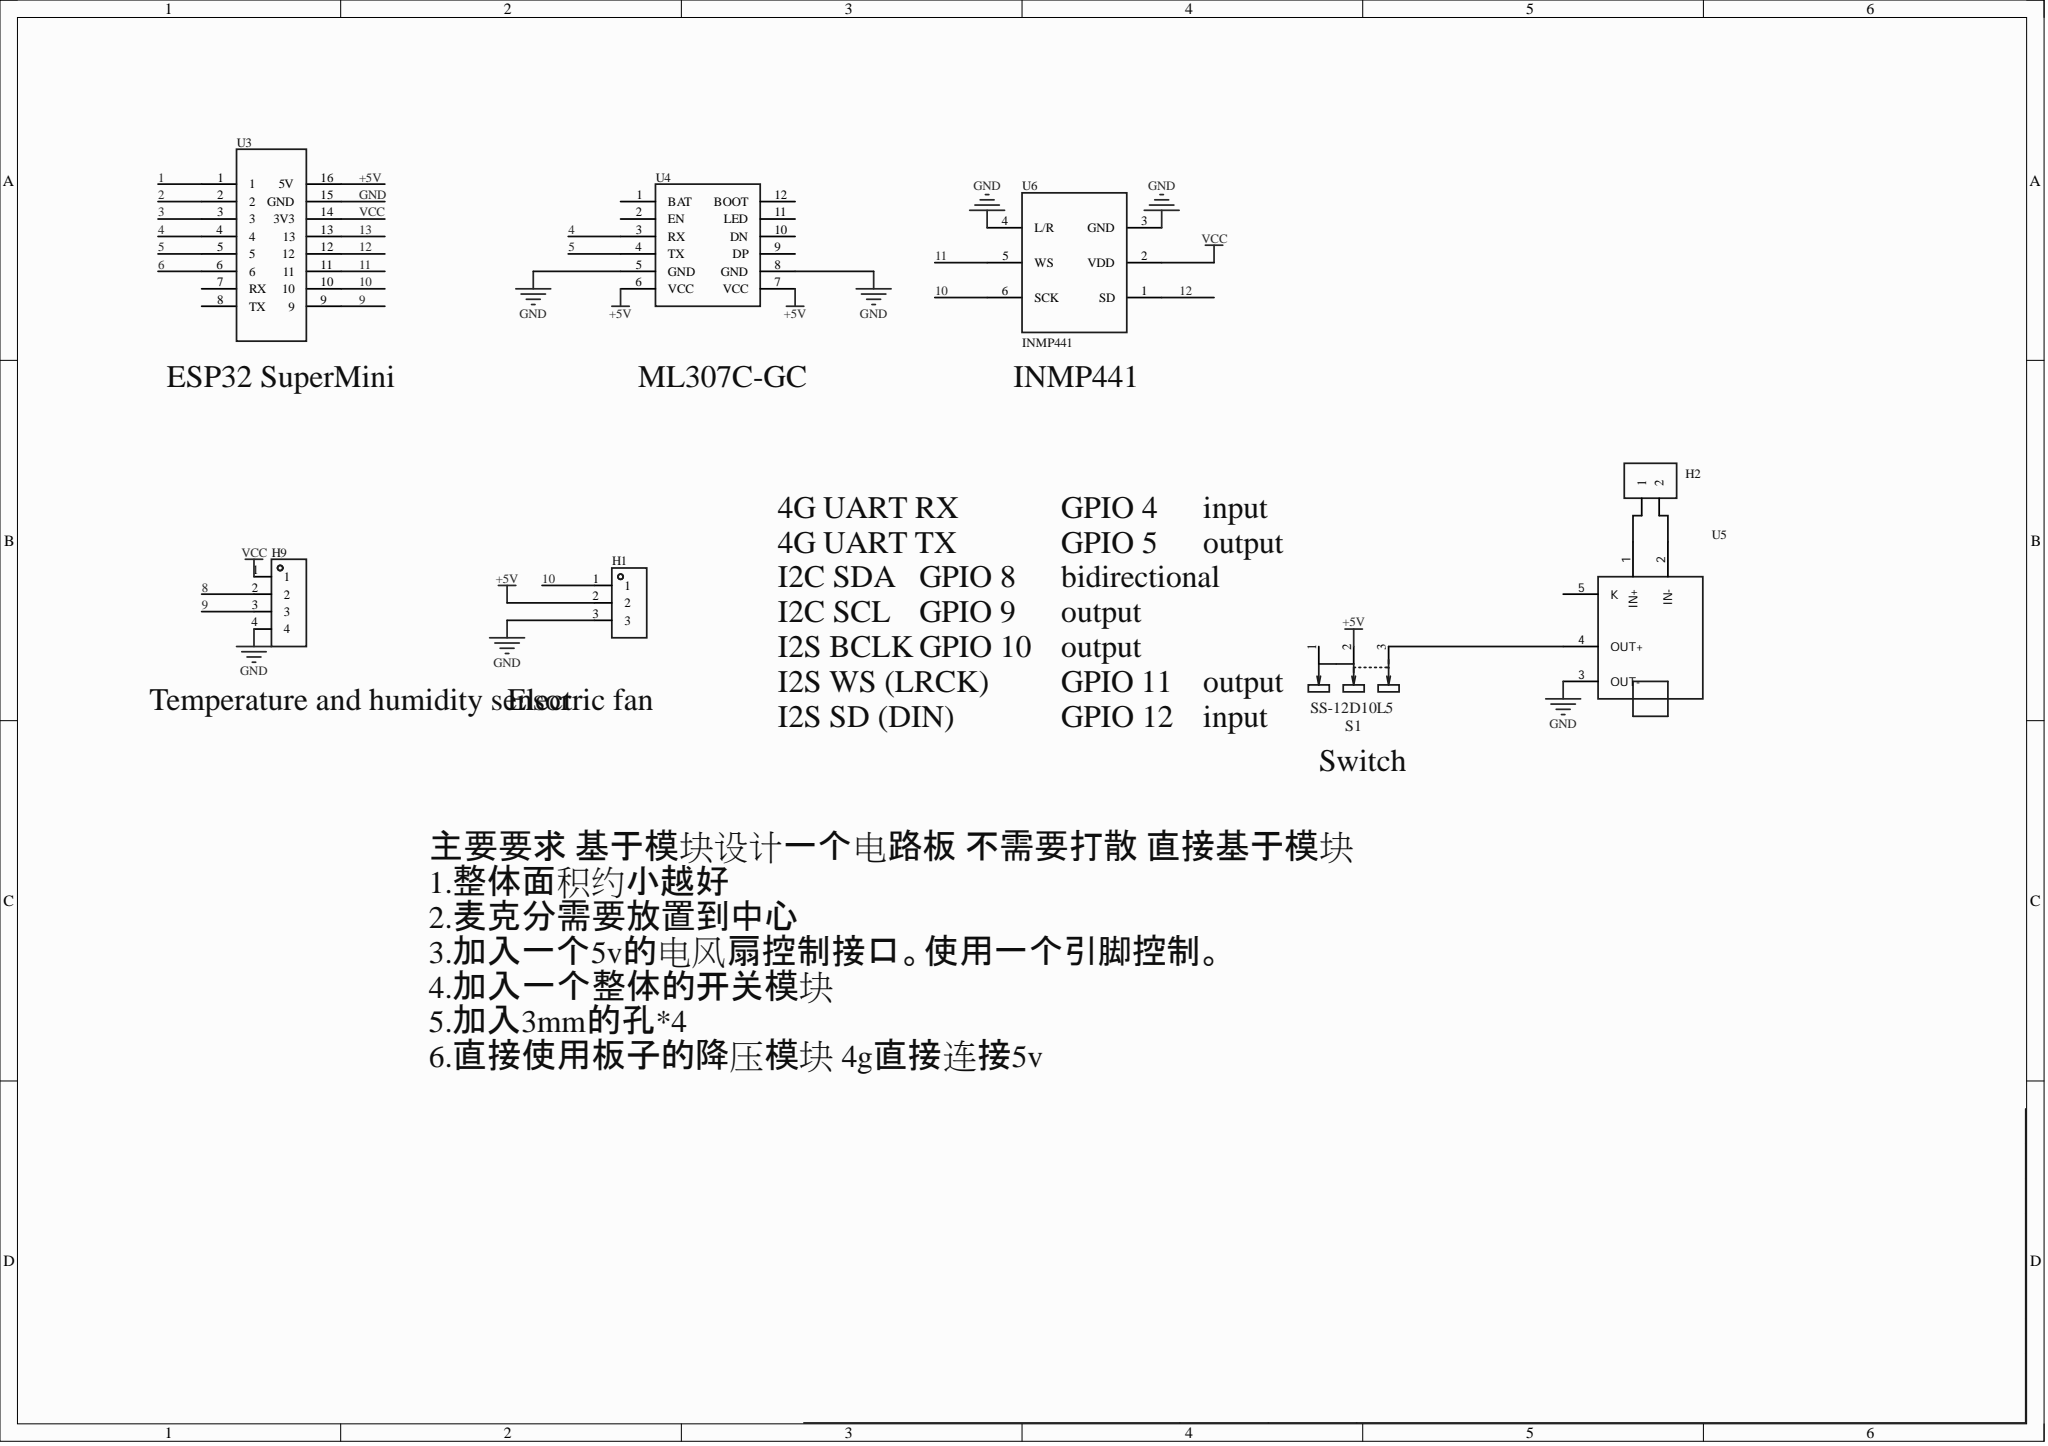Circuit board | Altium Designer | 8 parts | 12 nets
Bill of materials:
Comment,Description,Designator,Footprint,LibRef,Quantity
"","","H1","HDR-TH_3P-P2.54-V-M","HDR-M_2.54_1x3P","1"
"","","H2","HDR-TH_2P-P2.54-V-F","HDR-F_2.54_1x2P","1"
"","","H9","HDR-TH_4P-P2.54-V-F","HDR-F_2.54_1x4P","1"
"SS-12D10L5","","S1","SS-12D10L5","SS-12D10L5","1"
"","","U3","【封装Supermini】","ESP32 SuperMini","1"
"","","U4","ML307C-GC核心板","ML307C-GC核心板","1"
"","","U5","5V2A充放电一体模块","5V2A充放电一体模块","1"
"INMP441","","U6","INMP441","INMP441","1"
Netlist (Protel format):
[
H1
HDR-TH_3P-P2.54-V-M




]
[
H2
HDR-TH_2P-P2.54-V-F




]
[
H9
HDR-TH_4P-P2.54-V-F




]
[
S1
SS-12D10L5
SS-12D10L5



]
[
U3
【封装Supermini】




]
[
U4
ML307C-GC核心板




]
[
U5
5V2A充放电一体模块




]
[
U6
INMP441
INMP441



]
(
VCC
H9-1
U3-14
U6-2
)
(
NetS1_3
S1-3
U5-4
)
(
NetH2_2
H2-2
U5-2
)
(
NetH2_1
H2-1
U5-1
)
(
GND
H1-3
H9-4
U3-15
U4-5
U4-8
U5-3
U6-3
U6-4
)
(
+5V
H1-2
S1-2
U3-16
U4-6
U4-7
)
(
12
U3-12
U6-1
)
(
11
U3-11
U6-5
)
(
10
H1-1
U3-10
U6-6
)
(
9
H9-3
U3-9
)
(
5
U3-5
U4-4
)
(
4
U3-4
U4-3
)